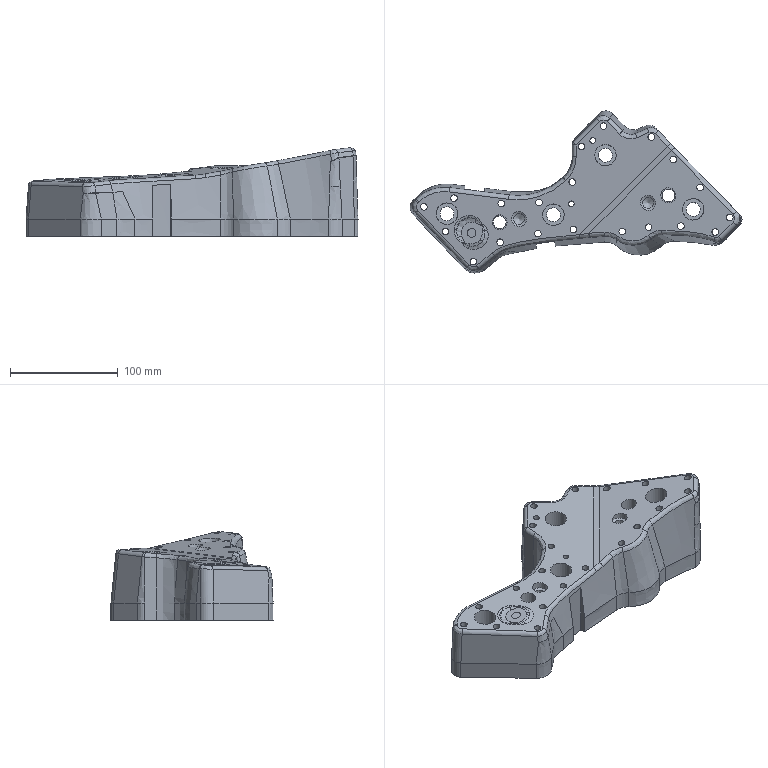Part | STEP file | gslz 2016.10.28-13_id1698_x_t | 1 solid | 226 faces | box 308.791 x 150.802 x 82.369 mm | volume 1185537 mm3 | spline 76 | cylinder 74 | plane 47 | other 24 | cone 4 | sphere 1 | commonest cylinder face diameters 10.3 x22 6.2 x20 7.5 x9 17.5 x5 13 x4 14 x4